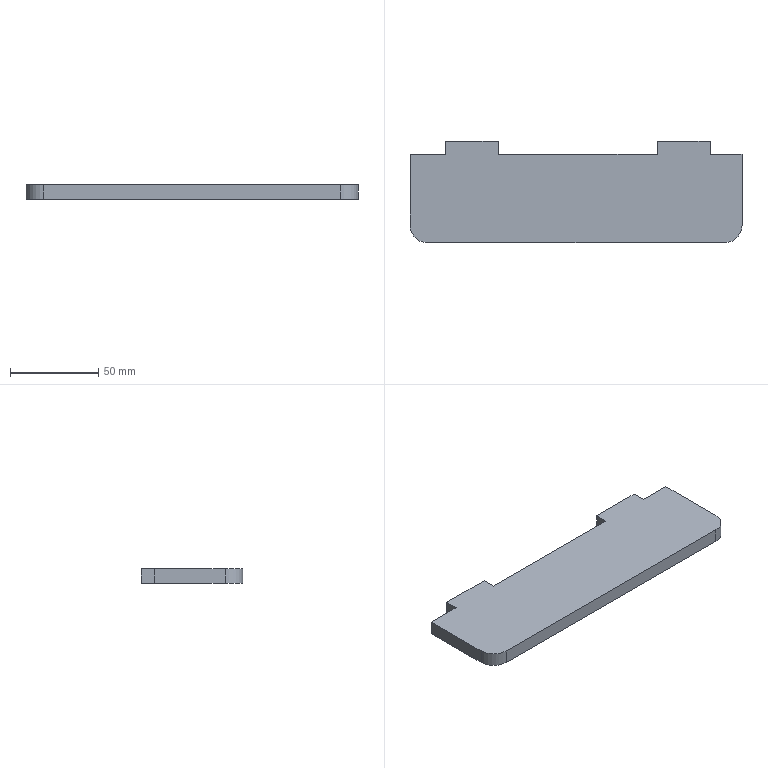Part | SolidWorks | features FlatPattern 1, SMBaseFlange 1, SheetMetal 1 | 1 solid | 16 faces | box 188 x 57.5 x 8 mm | volume 78457 mm3 | plane 14 | cylinder 2 | commonest cylinder face diameters 20 x2
STEP:
#1=CARTESIAN_POINT('',(-287.183,-291.5,0.));
#2=VERTEX_POINT('',#1);
#3=CARTESIAN_POINT('',(-307.183,-291.5,0.));
#4=VERTEX_POINT('',#3);
#5=CARTESIAN_POINT('',(-287.183,-291.5,0.));
#6=DIRECTION('',(-1.,0.,0.));
#7=VECTOR('',#6,1000.);
#8=LINE('',#5,#7);
#9=EDGE_CURVE('',#2,#4,#8,.T.);
#10=ORIENTED_EDGE('',*,*,#9,.F.);
#11=CARTESIAN_POINT('',(-287.183,-291.5,-8.));
#12=VERTEX_POINT('',#11);
#13=CARTESIAN_POINT('',(-287.183,-291.5,-8.));
#14=DIRECTION('',(0.,0.,1.));
#15=VECTOR('',#14,1000.);
#16=LINE('',#13,#15);
#17=EDGE_CURVE('',#12,#2,#16,.T.);
#18=ORIENTED_EDGE('',*,*,#17,.F.);
#19=CARTESIAN_POINT('',(-307.183,-291.5,-8.));
#20=VERTEX_POINT('',#19);
#21=CARTESIAN_POINT('',(-287.183,-291.5,-8.));
#22=DIRECTION('',(-1.,0.,0.));
#23=VECTOR('',#22,1000.);
#24=LINE('',#21,#23);
#25=EDGE_CURVE('',#12,#20,#24,.T.);
#26=ORIENTED_EDGE('',*,*,#25,.T.);
#27=CARTESIAN_POINT('',(-307.183,-291.5,-8.));
#28=DIRECTION('',(0.,0.,1.));
#29=VECTOR('',#28,1000.);
#30=LINE('',#27,#29);
#31=EDGE_CURVE('',#20,#4,#30,.T.);
#32=ORIENTED_EDGE('',*,*,#31,.T.);
#33=EDGE_LOOP('',(#10,#18,#26,#32));
#34=FACE_OUTER_BOUND('',#33,.T.);
#35=CARTESIAN_POINT('',(-287.183,-291.5,-8.));
#36=DIRECTION('',(0.,1.,0.));
#37=DIRECTION('',(0.,0.,1.));
#38=AXIS2_PLACEMENT_3D('',#35,#36,#37);
#39=PLANE('',#38);
#40=ADVANCED_FACE('',(#34),#39,.T.);
#41=CARTESIAN_POINT('',(-287.183,-284.,0.));
#42=VERTEX_POINT('',#41);
#43=CARTESIAN_POINT('',(-287.183,-284.,0.));
#44=DIRECTION('',(0.,-1.,0.));
#45=VECTOR('',#44,1000.);
#46=LINE('',#43,#45);
#47=EDGE_CURVE('',#42,#2,#46,.T.);
#48=ORIENTED_EDGE('',*,*,#47,.F.);
#49=CARTESIAN_POINT('',(-287.183,-284.,-8.));
#50=VERTEX_POINT('',#49);
#51=CARTESIAN_POINT('',(-287.183,-284.,-8.));
#52=DIRECTION('',(0.,0.,1.));
#53=VECTOR('',#52,1000.);
#54=LINE('',#51,#53);
#55=EDGE_CURVE('',#50,#42,#54,.T.);
#56=ORIENTED_EDGE('',*,*,#55,.F.);
#57=CARTESIAN_POINT('',(-287.183,-284.,-8.));
#58=DIRECTION('',(0.,-1.,0.));
#59=VECTOR('',#58,1000.);
#60=LINE('',#57,#59);
#61=EDGE_CURVE('',#50,#12,#60,.T.);
#62=ORIENTED_EDGE('',*,*,#61,.T.);
#63=ORIENTED_EDGE('',*,*,#17,.T.);
#64=EDGE_LOOP('',(#48,#56,#62,#63));
#65=FACE_OUTER_BOUND('',#64,.T.);
#66=CARTESIAN_POINT('',(-287.183,-284.,-8.));
#67=DIRECTION('',(-1.,0.,0.));
#68=DIRECTION('',(0.,0.,1.));
#69=AXIS2_PLACEMENT_3D('',#66,#67,#68);
#70=PLANE('',#69);
#71=ADVANCED_FACE('',(#65),#70,.T.);
#72=CARTESIAN_POINT('',(-257.183,-284.,0.));
#73=VERTEX_POINT('',#72);
#74=CARTESIAN_POINT('',(-257.183,-284.,0.));
#75=DIRECTION('',(-1.,0.,0.));
#76=VECTOR('',#75,1000.);
#77=LINE('',#74,#76);
#78=EDGE_CURVE('',#73,#42,#77,.T.);
#79=ORIENTED_EDGE('',*,*,#78,.F.);
#80=CARTESIAN_POINT('',(-257.183,-284.,-8.));
#81=VERTEX_POINT('',#80);
#82=CARTESIAN_POINT('',(-257.183,-284.,-8.));
#83=DIRECTION('',(0.,0.,1.));
#84=VECTOR('',#83,1000.);
#85=LINE('',#82,#84);
#86=EDGE_CURVE('',#81,#73,#85,.T.);
#87=ORIENTED_EDGE('',*,*,#86,.F.);
#88=CARTESIAN_POINT('',(-257.183,-284.,-8.));
#89=DIRECTION('',(-1.,0.,0.));
#90=VECTOR('',#89,1000.);
#91=LINE('',#88,#90);
#92=EDGE_CURVE('',#81,#50,#91,.T.);
#93=ORIENTED_EDGE('',*,*,#92,.T.);
#94=ORIENTED_EDGE('',*,*,#55,.T.);
#95=EDGE_LOOP('',(#79,#87,#93,#94));
#96=FACE_OUTER_BOUND('',#95,.T.);
#97=CARTESIAN_POINT('',(-257.183,-284.,-8.));
#98=DIRECTION('',(0.,1.,0.));
#99=DIRECTION('',(0.,0.,1.));
#100=AXIS2_PLACEMENT_3D('',#97,#98,#99);
#101=PLANE('',#100);
#102=ADVANCED_FACE('',(#96),#101,.T.);
#103=CARTESIAN_POINT('',(-257.183,-291.5,0.));
#104=VERTEX_POINT('',#103);
#105=CARTESIAN_POINT('',(-257.183,-291.5,0.));
#106=DIRECTION('',(0.,1.,0.));
#107=VECTOR('',#106,1000.);
#108=LINE('',#105,#107);
#109=EDGE_CURVE('',#104,#73,#108,.T.);
#110=ORIENTED_EDGE('',*,*,#109,.F.);
#111=CARTESIAN_POINT('',(-257.183,-291.5,-8.));
#112=VERTEX_POINT('',#111);
#113=CARTESIAN_POINT('',(-257.183,-291.5,-8.));
#114=DIRECTION('',(0.,0.,1.));
#115=VECTOR('',#114,1000.);
#116=LINE('',#113,#115);
#117=EDGE_CURVE('',#112,#104,#116,.T.);
#118=ORIENTED_EDGE('',*,*,#117,.F.);
#119=CARTESIAN_POINT('',(-257.183,-291.5,-8.));
#120=DIRECTION('',(0.,1.,0.));
#121=VECTOR('',#120,1000.);
#122=LINE('',#119,#121);
#123=EDGE_CURVE('',#112,#81,#122,.T.);
#124=ORIENTED_EDGE('',*,*,#123,.T.);
#125=ORIENTED_EDGE('',*,*,#86,.T.);
#126=EDGE_LOOP('',(#110,#118,#124,#125));
#127=FACE_OUTER_BOUND('',#126,.T.);
#128=CARTESIAN_POINT('',(-257.183,-291.5,-8.));
#129=DIRECTION('',(1.,0.,0.));
#130=DIRECTION('',(0.,0.,-1.));
#131=AXIS2_PLACEMENT_3D('',#128,#129,#130);
#132=PLANE('',#131);
#133=ADVANCED_FACE('',(#127),#132,.T.);
#134=CARTESIAN_POINT('',(-167.183,-291.5,0.));
#135=VERTEX_POINT('',#134);
#136=CARTESIAN_POINT('',(-167.183,-291.5,0.));
#137=DIRECTION('',(-1.,0.,0.));
#138=VECTOR('',#137,1000.);
#139=LINE('',#136,#138);
#140=EDGE_CURVE('',#135,#104,#139,.T.);
#141=ORIENTED_EDGE('',*,*,#140,.F.);
#142=CARTESIAN_POINT('',(-167.183,-291.5,-8.));
#143=VERTEX_POINT('',#142);
#144=CARTESIAN_POINT('',(-167.183,-291.5,-8.));
#145=DIRECTION('',(0.,0.,1.));
#146=VECTOR('',#145,1000.);
#147=LINE('',#144,#146);
#148=EDGE_CURVE('',#143,#135,#147,.T.);
#149=ORIENTED_EDGE('',*,*,#148,.F.);
#150=CARTESIAN_POINT('',(-167.183,-291.5,-8.));
#151=DIRECTION('',(-1.,0.,0.));
#152=VECTOR('',#151,1000.);
#153=LINE('',#150,#152);
#154=EDGE_CURVE('',#143,#112,#153,.T.);
#155=ORIENTED_EDGE('',*,*,#154,.T.);
#156=ORIENTED_EDGE('',*,*,#117,.T.);
#157=EDGE_LOOP('',(#141,#149,#155,#156));
#158=FACE_OUTER_BOUND('',#157,.T.);
#159=CARTESIAN_POINT('',(-167.183,-291.5,-8.));
#160=DIRECTION('',(0.,1.,0.));
#161=DIRECTION('',(0.,0.,1.));
#162=AXIS2_PLACEMENT_3D('',#159,#160,#161);
#163=PLANE('',#162);
#164=ADVANCED_FACE('',(#158),#163,.T.);
#165=CARTESIAN_POINT('',(-167.183,-284.,0.));
#166=VERTEX_POINT('',#165);
#167=CARTESIAN_POINT('',(-167.183,-284.,0.));
#168=DIRECTION('',(0.,-1.,0.));
#169=VECTOR('',#168,1000.);
#170=LINE('',#167,#169);
#171=EDGE_CURVE('',#166,#135,#170,.T.);
#172=ORIENTED_EDGE('',*,*,#171,.F.);
#173=CARTESIAN_POINT('',(-167.183,-284.,-8.));
#174=VERTEX_POINT('',#173);
#175=CARTESIAN_POINT('',(-167.183,-284.,-8.));
#176=DIRECTION('',(0.,0.,1.));
#177=VECTOR('',#176,1000.);
#178=LINE('',#175,#177);
#179=EDGE_CURVE('',#174,#166,#178,.T.);
#180=ORIENTED_EDGE('',*,*,#179,.F.);
#181=CARTESIAN_POINT('',(-167.183,-284.,-8.));
#182=DIRECTION('',(0.,-1.,0.));
#183=VECTOR('',#182,1000.);
#184=LINE('',#181,#183);
#185=EDGE_CURVE('',#174,#143,#184,.T.);
#186=ORIENTED_EDGE('',*,*,#185,.T.);
#187=ORIENTED_EDGE('',*,*,#148,.T.);
#188=EDGE_LOOP('',(#172,#180,#186,#187));
#189=FACE_OUTER_BOUND('',#188,.T.);
#190=CARTESIAN_POINT('',(-167.183,-284.,-8.));
#191=DIRECTION('',(-1.,0.,0.));
#192=DIRECTION('',(0.,0.,1.));
#193=AXIS2_PLACEMENT_3D('',#190,#191,#192);
#194=PLANE('',#193);
#195=ADVANCED_FACE('',(#189),#194,.T.);
#196=CARTESIAN_POINT('',(-137.183,-284.,0.));
#197=VERTEX_POINT('',#196);
#198=CARTESIAN_POINT('',(-137.183,-284.,0.));
#199=DIRECTION('',(-1.,0.,0.));
#200=VECTOR('',#199,1000.);
#201=LINE('',#198,#200);
#202=EDGE_CURVE('',#197,#166,#201,.T.);
#203=ORIENTED_EDGE('',*,*,#202,.F.);
#204=CARTESIAN_POINT('',(-137.183,-284.,-8.));
#205=VERTEX_POINT('',#204);
#206=CARTESIAN_POINT('',(-137.183,-284.,-8.));
#207=DIRECTION('',(0.,0.,1.));
#208=VECTOR('',#207,1000.);
#209=LINE('',#206,#208);
#210=EDGE_CURVE('',#205,#197,#209,.T.);
#211=ORIENTED_EDGE('',*,*,#210,.F.);
#212=CARTESIAN_POINT('',(-137.183,-284.,-8.));
#213=DIRECTION('',(-1.,0.,0.));
#214=VECTOR('',#213,1000.);
#215=LINE('',#212,#214);
#216=EDGE_CURVE('',#205,#174,#215,.T.);
#217=ORIENTED_EDGE('',*,*,#216,.T.);
#218=ORIENTED_EDGE('',*,*,#179,.T.);
#219=EDGE_LOOP('',(#203,#211,#217,#218));
#220=FACE_OUTER_BOUND('',#219,.T.);
#221=CARTESIAN_POINT('',(-137.183,-284.,-8.));
#222=DIRECTION('',(0.,1.,0.));
#223=DIRECTION('',(-1.,0.,0.));
#224=AXIS2_PLACEMENT_3D('',#221,#222,#223);
#225=PLANE('',#224);
#226=ADVANCED_FACE('',(#220),#225,.T.);
#227=CARTESIAN_POINT('',(-137.183,-291.5,0.));
#228=VERTEX_POINT('',#227);
#229=CARTESIAN_POINT('',(-137.183,-291.5,0.));
#230=DIRECTION('',(0.,1.,0.));
#231=VECTOR('',#230,1000.);
#232=LINE('',#229,#231);
#233=EDGE_CURVE('',#228,#197,#232,.T.);
#234=ORIENTED_EDGE('',*,*,#233,.F.);
#235=CARTESIAN_POINT('',(-137.183,-291.5,-8.));
#236=VERTEX_POINT('',#235);
#237=CARTESIAN_POINT('',(-137.183,-291.5,-8.));
#238=DIRECTION('',(0.,0.,1.));
#239=VECTOR('',#238,1000.);
#240=LINE('',#237,#239);
#241=EDGE_CURVE('',#236,#228,#240,.T.);
#242=ORIENTED_EDGE('',*,*,#241,.F.);
#243=CARTESIAN_POINT('',(-137.183,-291.5,-8.));
#244=DIRECTION('',(0.,1.,0.));
#245=VECTOR('',#244,1000.);
#246=LINE('',#243,#245);
#247=EDGE_CURVE('',#236,#205,#246,.T.);
#248=ORIENTED_EDGE('',*,*,#247,.T.);
#249=ORIENTED_EDGE('',*,*,#210,.T.);
#250=EDGE_LOOP('',(#234,#242,#248,#249));
#251=FACE_OUTER_BOUND('',#250,.T.);
#252=CARTESIAN_POINT('',(-137.183,-291.5,-8.));
#253=DIRECTION('',(1.,0.,0.));
#254=DIRECTION('',(0.,0.,-1.));
#255=AXIS2_PLACEMENT_3D('',#252,#253,#254);
#256=PLANE('',#255);
#257=ADVANCED_FACE('',(#251),#256,.T.);
#258=CARTESIAN_POINT('',(-119.183,-291.5,0.));
#259=VERTEX_POINT('',#258);
#260=CARTESIAN_POINT('',(-119.183,-291.5,0.));
#261=DIRECTION('',(-1.,0.,0.));
#262=VECTOR('',#261,1000.);
#263=LINE('',#260,#262);
#264=EDGE_CURVE('',#259,#228,#263,.T.);
#265=ORIENTED_EDGE('',*,*,#264,.F.);
#266=CARTESIAN_POINT('',(-119.183,-291.5,-8.));
#267=VERTEX_POINT('',#266);
#268=CARTESIAN_POINT('',(-119.183,-291.5,-8.));
#269=DIRECTION('',(0.,0.,1.));
#270=VECTOR('',#269,1000.);
#271=LINE('',#268,#270);
#272=EDGE_CURVE('',#267,#259,#271,.T.);
#273=ORIENTED_EDGE('',*,*,#272,.F.);
#274=CARTESIAN_POINT('',(-119.183,-291.5,-8.));
#275=DIRECTION('',(-1.,0.,0.));
#276=VECTOR('',#275,1000.);
#277=LINE('',#274,#276);
#278=EDGE_CURVE('',#267,#236,#277,.T.);
#279=ORIENTED_EDGE('',*,*,#278,.T.);
#280=ORIENTED_EDGE('',*,*,#241,.T.);
#281=EDGE_LOOP('',(#265,#273,#279,#280));
#282=FACE_OUTER_BOUND('',#281,.T.);
#283=CARTESIAN_POINT('',(-119.183,-291.5,-8.));
#284=DIRECTION('',(0.,1.,0.));
#285=DIRECTION('',(0.,0.,1.));
#286=AXIS2_PLACEMENT_3D('',#283,#284,#285);
#287=PLANE('',#286);
#288=ADVANCED_FACE('',(#282),#287,.T.);
#289=CARTESIAN_POINT('',(-119.183,-331.5,0.));
#290=VERTEX_POINT('',#289);
#291=CARTESIAN_POINT('',(-119.183,-331.5,0.));
#292=DIRECTION('',(0.,1.,0.));
#293=VECTOR('',#292,1000.);
#294=LINE('',#291,#293);
#295=EDGE_CURVE('',#290,#259,#294,.T.);
#296=ORIENTED_EDGE('',*,*,#295,.F.);
#297=CARTESIAN_POINT('',(-119.183,-331.5,-8.));
#298=VERTEX_POINT('',#297);
#299=CARTESIAN_POINT('',(-119.183,-331.5,-8.));
#300=DIRECTION('',(0.,0.,1.));
#301=VECTOR('',#300,1000.);
#302=LINE('',#299,#301);
#303=EDGE_CURVE('',#298,#290,#302,.T.);
#304=ORIENTED_EDGE('',*,*,#303,.F.);
#305=CARTESIAN_POINT('',(-119.183,-331.5,-8.));
#306=DIRECTION('',(0.,1.,0.));
#307=VECTOR('',#306,1000.);
#308=LINE('',#305,#307);
#309=EDGE_CURVE('',#298,#267,#308,.T.);
#310=ORIENTED_EDGE('',*,*,#309,.T.);
#311=ORIENTED_EDGE('',*,*,#272,.T.);
#312=EDGE_LOOP('',(#296,#304,#310,#311));
#313=FACE_OUTER_BOUND('',#312,.T.);
#314=CARTESIAN_POINT('',(-119.183,-331.5,-8.));
#315=DIRECTION('',(1.,0.,0.));
#316=DIRECTION('',(0.,0.,-1.));
#317=AXIS2_PLACEMENT_3D('',#314,#315,#316);
#318=PLANE('',#317);
#319=ADVANCED_FACE('',(#313),#318,.T.);
#320=CARTESIAN_POINT('',(-129.183,-341.5,0.));
#321=VERTEX_POINT('',#320);
#322=CARTESIAN_POINT('',(-129.183,-331.5,0.));
#323=DIRECTION('',(0.,0.,1.));
#324=DIRECTION('',(1.,0.,0.));
#325=AXIS2_PLACEMENT_3D('',#322,#323,#324);
#326=CIRCLE('',#325,10.);
#327=EDGE_CURVE('',#321,#290,#326,.T.);
#328=ORIENTED_EDGE('',*,*,#327,.F.);
#329=CARTESIAN_POINT('',(-129.183,-341.5,-8.));
#330=VERTEX_POINT('',#329);
#331=CARTESIAN_POINT('',(-129.183,-341.5,-8.));
#332=DIRECTION('',(0.,0.,1.));
#333=VECTOR('',#332,1000.);
#334=LINE('',#331,#333);
#335=EDGE_CURVE('',#330,#321,#334,.T.);
#336=ORIENTED_EDGE('',*,*,#335,.F.);
#337=CARTESIAN_POINT('',(-129.183,-331.5,-8.));
#338=DIRECTION('',(0.,0.,1.));
#339=DIRECTION('',(1.,0.,0.));
#340=AXIS2_PLACEMENT_3D('',#337,#338,#339);
#341=CIRCLE('',#340,10.);
#342=EDGE_CURVE('',#330,#298,#341,.T.);
#343=ORIENTED_EDGE('',*,*,#342,.T.);
#344=ORIENTED_EDGE('',*,*,#303,.T.);
#345=EDGE_LOOP('',(#328,#336,#343,#344));
#346=FACE_OUTER_BOUND('',#345,.T.);
#347=CARTESIAN_POINT('',(-129.183,-331.5,-8.));
#348=DIRECTION('',(0.,0.,1.));
#349=DIRECTION('',(1.,0.,0.));
#350=AXIS2_PLACEMENT_3D('',#347,#348,#349);
#351=CYLINDRICAL_SURFACE('',#350,10.);
#352=ADVANCED_FACE('',(#346),#351,.T.);
#353=CARTESIAN_POINT('',(-297.183,-341.5,0.));
#354=VERTEX_POINT('',#353);
#355=CARTESIAN_POINT('',(-297.183,-341.5,0.));
#356=DIRECTION('',(1.,0.,0.));
#357=VECTOR('',#356,1000.);
#358=LINE('',#355,#357);
#359=EDGE_CURVE('',#354,#321,#358,.T.);
#360=ORIENTED_EDGE('',*,*,#359,.F.);
#361=CARTESIAN_POINT('',(-297.183,-341.5,-8.));
#362=VERTEX_POINT('',#361);
#363=CARTESIAN_POINT('',(-297.183,-341.5,-8.));
#364=DIRECTION('',(0.,0.,1.));
#365=VECTOR('',#364,1000.);
#366=LINE('',#363,#365);
#367=EDGE_CURVE('',#362,#354,#366,.T.);
#368=ORIENTED_EDGE('',*,*,#367,.F.);
#369=CARTESIAN_POINT('',(-297.183,-341.5,-8.));
#370=DIRECTION('',(1.,0.,0.));
#371=VECTOR('',#370,1000.);
#372=LINE('',#369,#371);
#373=EDGE_CURVE('',#362,#330,#372,.T.);
#374=ORIENTED_EDGE('',*,*,#373,.T.);
#375=ORIENTED_EDGE('',*,*,#335,.T.);
#376=EDGE_LOOP('',(#360,#368,#374,#375));
#377=FACE_OUTER_BOUND('',#376,.T.);
#378=CARTESIAN_POINT('',(-297.183,-341.5,-8.));
#379=DIRECTION('',(0.,-1.,0.));
#380=DIRECTION('',(0.,0.,-1.));
#381=AXIS2_PLACEMENT_3D('',#378,#379,#380);
#382=PLANE('',#381);
#383=ADVANCED_FACE('',(#377),#382,.T.);
#384=CARTESIAN_POINT('',(-307.183,-331.5,0.));
#385=VERTEX_POINT('',#384);
#386=CARTESIAN_POINT('',(-297.183,-331.5,0.));
#387=DIRECTION('',(0.,0.,1.));
#388=DIRECTION('',(1.,0.,0.));
#389=AXIS2_PLACEMENT_3D('',#386,#387,#388);
#390=CIRCLE('',#389,10.);
#391=EDGE_CURVE('',#385,#354,#390,.T.);
#392=ORIENTED_EDGE('',*,*,#391,.F.);
#393=CARTESIAN_POINT('',(-307.183,-331.5,-8.));
#394=VERTEX_POINT('',#393);
#395=CARTESIAN_POINT('',(-307.183,-331.5,-8.));
#396=DIRECTION('',(0.,0.,1.));
#397=VECTOR('',#396,1000.);
#398=LINE('',#395,#397);
#399=EDGE_CURVE('',#394,#385,#398,.T.);
#400=ORIENTED_EDGE('',*,*,#399,.F.);
#401=CARTESIAN_POINT('',(-297.183,-331.5,-8.));
#402=DIRECTION('',(0.,0.,1.));
#403=DIRECTION('',(1.,0.,0.));
#404=AXIS2_PLACEMENT_3D('',#401,#402,#403);
#405=CIRCLE('',#404,10.);
#406=EDGE_CURVE('',#394,#362,#405,.T.);
#407=ORIENTED_EDGE('',*,*,#406,.T.);
#408=ORIENTED_EDGE('',*,*,#367,.T.);
#409=EDGE_LOOP('',(#392,#400,#407,#408));
#410=FACE_OUTER_BOUND('',#409,.T.);
#411=CARTESIAN_POINT('',(-297.183,-331.5,-8.));
#412=DIRECTION('',(0.,0.,1.));
#413=DIRECTION('',(1.,0.,0.));
#414=AXIS2_PLACEMENT_3D('',#411,#412,#413);
#415=CYLINDRICAL_SURFACE('',#414,10.);
#416=ADVANCED_FACE('',(#410),#415,.T.);
#417=CARTESIAN_POINT('',(-307.183,-291.5,0.));
#418=DIRECTION('',(0.,-1.,0.));
#419=VECTOR('',#418,1000.);
#420=LINE('',#417,#419);
#421=EDGE_CURVE('',#4,#385,#420,.T.);
#422=ORIENTED_EDGE('',*,*,#421,.F.);
#423=ORIENTED_EDGE('',*,*,#31,.F.);
#424=CARTESIAN_POINT('',(-307.183,-291.5,-8.));
#425=DIRECTION('',(0.,-1.,0.));
#426=VECTOR('',#425,1000.);
#427=LINE('',#424,#426);
#428=EDGE_CURVE('',#20,#394,#427,.T.);
#429=ORIENTED_EDGE('',*,*,#428,.T.);
#430=ORIENTED_EDGE('',*,*,#399,.T.);
#431=EDGE_LOOP('',(#422,#423,#429,#430));
#432=FACE_OUTER_BOUND('',#431,.T.);
#433=CARTESIAN_POINT('',(-307.183,-291.5,-8.));
#434=DIRECTION('',(-1.,0.,0.));
#435=DIRECTION('',(0.,0.,1.));
#436=AXIS2_PLACEMENT_3D('',#433,#434,#435);
#437=PLANE('',#436);
#438=ADVANCED_FACE('',(#432),#437,.T.);
#439=ORIENTED_EDGE('',*,*,#25,.F.);
#440=ORIENTED_EDGE('',*,*,#61,.F.);
#441=ORIENTED_EDGE('',*,*,#92,.F.);
#442=ORIENTED_EDGE('',*,*,#123,.F.);
#443=ORIENTED_EDGE('',*,*,#154,.F.);
#444=ORIENTED_EDGE('',*,*,#185,.F.);
#445=ORIENTED_EDGE('',*,*,#216,.F.);
#446=ORIENTED_EDGE('',*,*,#247,.F.);
#447=ORIENTED_EDGE('',*,*,#278,.F.);
#448=ORIENTED_EDGE('',*,*,#309,.F.);
#449=ORIENTED_EDGE('',*,*,#342,.F.);
#450=ORIENTED_EDGE('',*,*,#373,.F.);
#451=ORIENTED_EDGE('',*,*,#406,.F.);
#452=ORIENTED_EDGE('',*,*,#428,.F.);
#453=EDGE_LOOP('',(#439,#440,#441,#442,#443,#444,#445,#446,#447,#448,#449,#450,#451,#452));
#454=FACE_OUTER_BOUND('',#453,.T.);
#455=CARTESIAN_POINT('',(-297.183,-331.5,-8.));
#456=DIRECTION('',(0.,0.,1.));
#457=DIRECTION('',(1.,0.,0.));
#458=AXIS2_PLACEMENT_3D('',#455,#456,#457);
#459=PLANE('',#458);
#460=ADVANCED_FACE('',(#454),#459,.F.);
#461=ORIENTED_EDGE('',*,*,#9,.T.);
#462=ORIENTED_EDGE('',*,*,#421,.T.);
#463=ORIENTED_EDGE('',*,*,#391,.T.);
#464=ORIENTED_EDGE('',*,*,#359,.T.);
#465=ORIENTED_EDGE('',*,*,#327,.T.);
#466=ORIENTED_EDGE('',*,*,#295,.T.);
#467=ORIENTED_EDGE('',*,*,#264,.T.);
#468=ORIENTED_EDGE('',*,*,#233,.T.);
#469=ORIENTED_EDGE('',*,*,#202,.T.);
#470=ORIENTED_EDGE('',*,*,#171,.T.);
#471=ORIENTED_EDGE('',*,*,#140,.T.);
#472=ORIENTED_EDGE('',*,*,#109,.T.);
#473=ORIENTED_EDGE('',*,*,#78,.T.);
#474=ORIENTED_EDGE('',*,*,#47,.T.);
#475=EDGE_LOOP('',(#461,#462,#463,#464,#465,#466,#467,#468,#469,#470,#471,#472,#473,#474));
#476=FACE_OUTER_BOUND('',#475,.T.);
#477=CARTESIAN_POINT('',(-297.183,-331.5,0.));
#478=DIRECTION('',(0.,0.,1.));
#479=DIRECTION('',(1.,0.,0.));
#480=AXIS2_PLACEMENT_3D('',#477,#478,#479);
#481=PLANE('',#480);
#482=ADVANCED_FACE('',(#476),#481,.T.);
#483=CLOSED_SHELL('',(#40,#71,#102,#133,#164,#195,#226,#257,#288,#319,#352,#383,#416,#438,#460,#482));
#484=MANIFOLD_SOLID_BREP('',#483);
#485=CARTESIAN_POINT('',(0.,0.,0.));
#486=DIRECTION('',(0.,0.,1.));
#487=DIRECTION('',(1.,0.,0.));
#488=AXIS2_PLACEMENT_3D('',#485,#486,#487);
#489=(LENGTH_UNIT()NAMED_UNIT(*)SI_UNIT(.MILLI.,.METRE.));
#490=UNCERTAINTY_MEASURE_WITH_UNIT(LENGTH_MEASURE(0.00001),#489,'','');
#491=(NAMED_UNIT(*)PLANE_ANGLE_UNIT()SI_UNIT($,.RADIAN.));
#492=(NAMED_UNIT(*)SI_UNIT($,.STERADIAN.)SOLID_ANGLE_UNIT());
#493=(GEOMETRIC_REPRESENTATION_CONTEXT(3)GLOBAL_UNCERTAINTY_ASSIGNED_CONTEXT((#490))GLOBAL_UNIT_ASSIGNED_CONTEXT((#489,#491,#492))REPRESENTATION_CONTEXT('',''));
#494=ADVANCED_BREP_SHAPE_REPRESENTATION('',(#484,#488),#493);